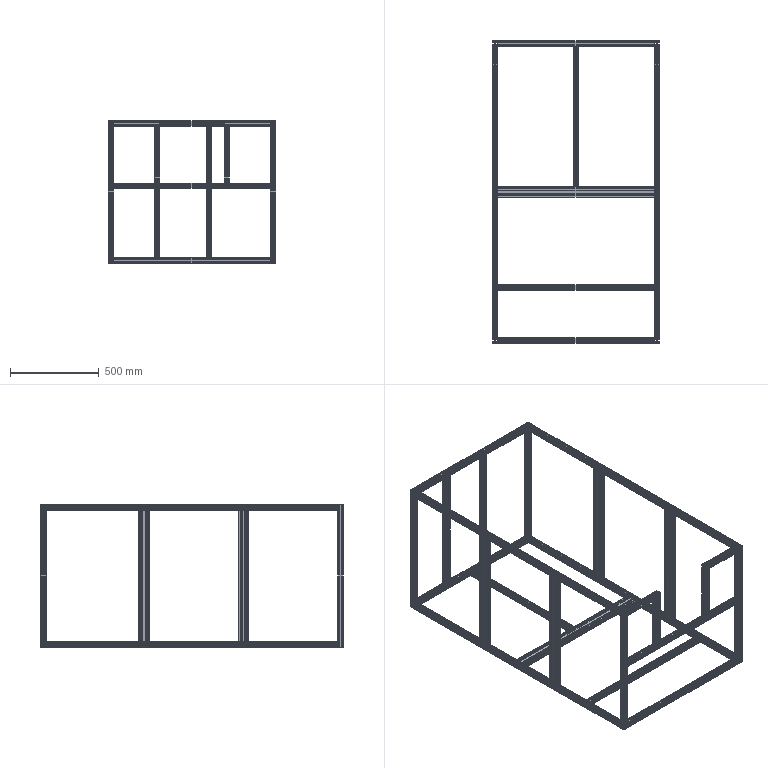Part | STEP file | 001-002-Aluminium profile frame_default<machined> | 25 solids | 1928 faces | box 940 x 1700 x 800 mm | volume 8888150 mm3 | plane 1530 | cylinder 398 | commonest cylinder face diameters 3 x260 5.3 x40 6.8 x40 24 x37 5 x21